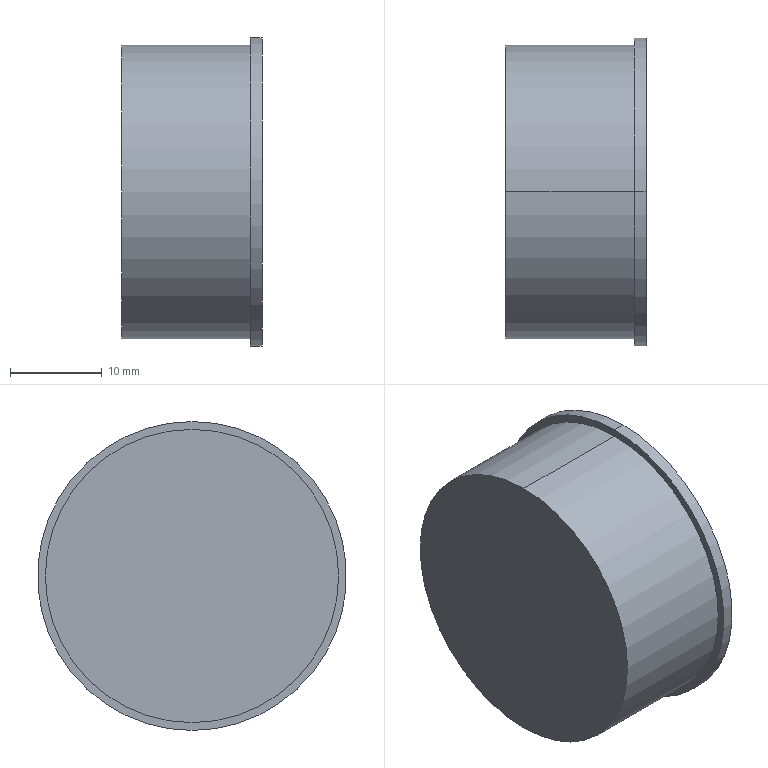Part | SolidWorks | features BaseBody 1 | 1 solid | 13 faces | box 15.3 x 33.7 x 33.7 mm | volume 12319 mm3 | cylinder 6 | cone 4 | plane 3 | commonest cylinder face diameters 4.5 x2 32 x2 33.7 x2
STEP:
#1=CARTESIAN_POINT('',(-209.5,-84.,82.771));
#2=VERTEX_POINT('',#1);
#3=CARTESIAN_POINT('',(-209.5,-84.,116.471));
#4=VERTEX_POINT('',#3);
#5=CARTESIAN_POINT('',(-209.5,-84.,99.621));
#6=DIRECTION('',(1.,0.,0.));
#7=DIRECTION('',(0.,0.,-1.));
#8=AXIS2_PLACEMENT_3D('',#5,#6,#7);
#9=CIRCLE('',#8,16.85);
#10=EDGE_CURVE('',#2,#4,#9,.T.);
#11=ORIENTED_EDGE('',*,*,#10,.T.);
#12=CARTESIAN_POINT('',(-208.2,-84.,116.471));
#13=VERTEX_POINT('',#12);
#14=CARTESIAN_POINT('',(-209.5,-84.,116.471));
#15=DIRECTION('',(1.,0.,0.));
#16=VECTOR('',#15,1000.);
#17=LINE('',#14,#16);
#18=EDGE_CURVE('',#4,#13,#17,.T.);
#19=ORIENTED_EDGE('',*,*,#18,.T.);
#20=CARTESIAN_POINT('',(-208.2,-84.,82.771));
#21=VERTEX_POINT('',#20);
#22=CARTESIAN_POINT('',(-208.2,-84.,99.621));
#23=DIRECTION('',(-1.,0.,0.));
#24=DIRECTION('',(0.,0.,-1.));
#25=AXIS2_PLACEMENT_3D('',#22,#23,#24);
#26=CIRCLE('',#25,16.85);
#27=EDGE_CURVE('',#13,#21,#26,.T.);
#28=ORIENTED_EDGE('',*,*,#27,.T.);
#29=CARTESIAN_POINT('',(-209.5,-84.,82.771));
#30=DIRECTION('',(1.,0.,0.));
#31=VECTOR('',#30,1000.);
#32=LINE('',#29,#31);
#33=EDGE_CURVE('',#2,#21,#32,.T.);
#34=ORIENTED_EDGE('',*,*,#33,.F.);
#35=EDGE_LOOP('',(#11,#19,#28,#34));
#36=FACE_OUTER_BOUND('',#35,.T.);
#37=CARTESIAN_POINT('',(-209.5,-84.,99.621));
#38=DIRECTION('',(1.,0.,0.));
#39=DIRECTION('',(0.,0.,-1.));
#40=AXIS2_PLACEMENT_3D('',#37,#38,#39);
#41=CYLINDRICAL_SURFACE('',#40,16.85);
#42=ADVANCED_FACE('',(#36),#41,.T.);
#43=CARTESIAN_POINT('',(-209.914,-86.25,99.621));
#44=VERTEX_POINT('',#43);
#45=CARTESIAN_POINT('',(-209.914,-84.,97.371));
#46=VERTEX_POINT('',#45);
#47=CARTESIAN_POINT('',(-209.914,-84.,99.621));
#48=DIRECTION('',(1.,0.,0.));
#49=DIRECTION('',(0.,0.3818,-0.9242));
#50=AXIS2_PLACEMENT_3D('',#47,#48,#49);
#51=CIRCLE('',#50,2.25);
#52=EDGE_CURVE('',#44,#46,#51,.T.);
#53=ORIENTED_EDGE('',*,*,#52,.F.);
#54=CARTESIAN_POINT('',(-208.2,-87.964,99.621));
#55=VERTEX_POINT('',#54);
#56=CARTESIAN_POINT('',(-208.2,-87.964,99.621));
#57=DIRECTION('',(0.7071,-0.7071,0.));
#58=VECTOR('',#57,1000.);
#59=LINE('',#56,#58);
#60=EDGE_CURVE('',#44,#55,#59,.T.);
#61=ORIENTED_EDGE('',*,*,#60,.T.);
#62=CARTESIAN_POINT('',(-208.2,-80.036,99.621));
#63=VERTEX_POINT('',#62);
#64=CARTESIAN_POINT('',(-208.2,-84.,99.621));
#65=DIRECTION('',(1.,0.,0.));
#66=DIRECTION('',(0.,1.,0.));
#67=AXIS2_PLACEMENT_3D('',#64,#65,#66);
#68=CIRCLE('',#67,3.964);
#69=EDGE_CURVE('',#55,#63,#68,.T.);
#70=ORIENTED_EDGE('',*,*,#69,.T.);
#71=CARTESIAN_POINT('',(-209.914,-81.75,99.621));
#72=VERTEX_POINT('',#71);
#73=CARTESIAN_POINT('',(-208.2,-80.036,99.621));
#74=DIRECTION('',(0.7071,0.7071,0.));
#75=VECTOR('',#74,1000.);
#76=LINE('',#73,#75);
#77=EDGE_CURVE('',#72,#63,#76,.T.);
#78=ORIENTED_EDGE('',*,*,#77,.F.);
#79=CARTESIAN_POINT('',(-209.914,-84.,99.621));
#80=DIRECTION('',(1.,0.,0.));
#81=DIRECTION('',(0.,0.3818,-0.9242));
#82=AXIS2_PLACEMENT_3D('',#79,#80,#81);
#83=CIRCLE('',#82,2.25);
#84=EDGE_CURVE('',#46,#72,#83,.T.);
#85=ORIENTED_EDGE('',*,*,#84,.F.);
#86=EDGE_LOOP('',(#53,#61,#70,#78,#85));
#87=FACE_OUTER_BOUND('',#86,.T.);
#88=CARTESIAN_POINT('',(-208.2,-84.,99.621));
#89=DIRECTION('',(1.,0.,0.));
#90=DIRECTION('',(0.,1.,0.));
#91=AXIS2_PLACEMENT_3D('',#88,#89,#90);
#92=CONICAL_SURFACE('',#91,3.964,0.7854);
#93=ADVANCED_FACE('',(#87),#92,.F.);
#94=CARTESIAN_POINT('',(-212.43,-84.,101.871));
#95=VERTEX_POINT('',#94);
#96=CARTESIAN_POINT('',(-212.43,-84.,97.371));
#97=VERTEX_POINT('',#96);
#98=CARTESIAN_POINT('',(-212.43,-84.,99.621));
#99=DIRECTION('',(1.,0.,0.));
#100=DIRECTION('',(0.,0.,-1.));
#101=AXIS2_PLACEMENT_3D('',#98,#99,#100);
#102=CIRCLE('',#101,2.25);
#103=EDGE_CURVE('',#95,#97,#102,.T.);
#104=ORIENTED_EDGE('',*,*,#103,.F.);
#105=CARTESIAN_POINT('',(-209.914,-84.,101.871));
#106=VERTEX_POINT('',#105);
#107=CARTESIAN_POINT('',(-208.2,-84.,101.871));
#108=DIRECTION('',(1.,0.,0.));
#109=VECTOR('',#108,1000.);
#110=LINE('',#107,#109);
#111=EDGE_CURVE('',#95,#106,#110,.T.);
#112=ORIENTED_EDGE('',*,*,#111,.T.);
#113=CARTESIAN_POINT('',(-209.914,-84.,99.621));
#114=DIRECTION('',(1.,0.,0.));
#115=DIRECTION('',(0.,0.3818,-0.9242));
#116=AXIS2_PLACEMENT_3D('',#113,#114,#115);
#117=CIRCLE('',#116,2.25);
#118=EDGE_CURVE('',#106,#44,#117,.T.);
#119=ORIENTED_EDGE('',*,*,#118,.T.);
#120=ORIENTED_EDGE('',*,*,#52,.T.);
#121=CARTESIAN_POINT('',(-208.2,-84.,97.371));
#122=DIRECTION('',(1.,0.,0.));
#123=VECTOR('',#122,1000.);
#124=LINE('',#121,#123);
#125=EDGE_CURVE('',#97,#46,#124,.T.);
#126=ORIENTED_EDGE('',*,*,#125,.F.);
#127=EDGE_LOOP('',(#104,#112,#119,#120,#126));
#128=FACE_OUTER_BOUND('',#127,.T.);
#129=CARTESIAN_POINT('',(-208.2,-84.,99.621));
#130=DIRECTION('',(1.,0.,0.));
#131=DIRECTION('',(0.,0.,-1.));
#132=AXIS2_PLACEMENT_3D('',#129,#130,#131);
#133=CYLINDRICAL_SURFACE('',#132,2.25);
#134=ADVANCED_FACE('',(#128),#133,.F.);
#135=CARTESIAN_POINT('',(-223.5,-84.,83.621));
#136=VERTEX_POINT('',#135);
#137=CARTESIAN_POINT('',(-223.5,-84.,115.621));
#138=VERTEX_POINT('',#137);
#139=CARTESIAN_POINT('',(-223.5,-84.,99.621));
#140=DIRECTION('',(1.,0.,0.));
#141=DIRECTION('',(0.,0.,-1.));
#142=AXIS2_PLACEMENT_3D('',#139,#140,#141);
#143=CIRCLE('',#142,16.);
#144=EDGE_CURVE('',#136,#138,#143,.T.);
#145=ORIENTED_EDGE('',*,*,#144,.T.);
#146=CARTESIAN_POINT('',(-209.5,-84.,115.621));
#147=VERTEX_POINT('',#146);
#148=CARTESIAN_POINT('',(-223.5,-84.,115.621));
#149=DIRECTION('',(1.,0.,0.));
#150=VECTOR('',#149,1000.);
#151=LINE('',#148,#150);
#152=EDGE_CURVE('',#138,#147,#151,.T.);
#153=ORIENTED_EDGE('',*,*,#152,.T.);
#154=CARTESIAN_POINT('',(-209.5,-84.,83.621));
#155=VERTEX_POINT('',#154);
#156=CARTESIAN_POINT('',(-209.5,-84.,99.621));
#157=DIRECTION('',(1.,0.,0.));
#158=DIRECTION('',(0.,0.,-1.));
#159=AXIS2_PLACEMENT_3D('',#156,#157,#158);
#160=CIRCLE('',#159,16.);
#161=EDGE_CURVE('',#155,#147,#160,.T.);
#162=ORIENTED_EDGE('',*,*,#161,.F.);
#163=CARTESIAN_POINT('',(-223.5,-84.,83.621));
#164=DIRECTION('',(1.,0.,0.));
#165=VECTOR('',#164,1000.);
#166=LINE('',#163,#165);
#167=EDGE_CURVE('',#136,#155,#166,.T.);
#168=ORIENTED_EDGE('',*,*,#167,.F.);
#169=EDGE_LOOP('',(#145,#153,#162,#168));
#170=FACE_OUTER_BOUND('',#169,.T.);
#171=CARTESIAN_POINT('',(-223.5,-84.,99.621));
#172=DIRECTION('',(1.,0.,0.));
#173=DIRECTION('',(0.,0.,-1.));
#174=AXIS2_PLACEMENT_3D('',#171,#172,#173);
#175=CYLINDRICAL_SURFACE('',#174,16.);
#176=ADVANCED_FACE('',(#170),#175,.T.);
#177=CARTESIAN_POINT('',(-213.782,-84.,99.621));
#178=VERTEX_POINT('',#177);
#179=CARTESIAN_POINT('',(-212.43,-84.,97.371));
#180=DIRECTION('',(0.515,0.,-0.8572));
#181=VECTOR('',#180,1000.);
#182=LINE('',#179,#181);
#183=EDGE_CURVE('',#178,#97,#182,.T.);
#184=ORIENTED_EDGE('',*,*,#183,.F.);
#185=CARTESIAN_POINT('',(-212.43,-84.,101.871));
#186=DIRECTION('',(0.515,0.,0.8572));
#187=VECTOR('',#186,1000.);
#188=LINE('',#185,#187);
#189=EDGE_CURVE('',#178,#95,#188,.T.);
#190=ORIENTED_EDGE('',*,*,#189,.T.);
#191=ORIENTED_EDGE('',*,*,#103,.T.);
#192=EDGE_LOOP('',(#184,#190,#191));
#193=FACE_OUTER_BOUND('',#192,.T.);
#194=CARTESIAN_POINT('',(-212.43,-84.,99.621));
#195=DIRECTION('',(1.,0.,0.));
#196=DIRECTION('',(0.,0.,-1.));
#197=AXIS2_PLACEMENT_3D('',#194,#195,#196);
#198=CONICAL_SURFACE('',#197,2.25,1.03);
#199=ADVANCED_FACE('',(#193),#198,.F.);
#200=CARTESIAN_POINT('',(-208.2,-84.,99.621));
#201=DIRECTION('',(-1.,0.,0.));
#202=DIRECTION('',(0.,0.,-1.));
#203=AXIS2_PLACEMENT_3D('',#200,#201,#202);
#204=CIRCLE('',#203,16.85);
#205=EDGE_CURVE('',#21,#13,#204,.T.);
#206=ORIENTED_EDGE('',*,*,#205,.F.);
#207=ORIENTED_EDGE('',*,*,#27,.F.);
#208=EDGE_LOOP('',(#206,#207));
#209=FACE_OUTER_BOUND('',#208,.T.);
#210=CARTESIAN_POINT('',(-208.2,-84.,99.621));
#211=DIRECTION('',(1.,0.,0.));
#212=DIRECTION('',(0.,1.,0.));
#213=AXIS2_PLACEMENT_3D('',#210,#211,#212);
#214=CIRCLE('',#213,3.964);
#215=EDGE_CURVE('',#63,#55,#214,.T.);
#216=ORIENTED_EDGE('',*,*,#215,.F.);
#217=ORIENTED_EDGE('',*,*,#69,.F.);
#218=EDGE_LOOP('',(#216,#217));
#219=FACE_BOUND('',#218,.T.);
#220=CARTESIAN_POINT('',(-208.2,-84.,99.621));
#221=DIRECTION('',(-1.,0.,0.));
#222=DIRECTION('',(0.,0.,1.));
#223=AXIS2_PLACEMENT_3D('',#220,#221,#222);
#224=PLANE('',#223);
#225=ADVANCED_FACE('',(#209,#219),#224,.F.);
#226=ORIENTED_EDGE('',*,*,#18,.F.);
#227=CARTESIAN_POINT('',(-209.5,-84.,99.621));
#228=DIRECTION('',(1.,0.,0.));
#229=DIRECTION('',(0.,0.,-1.));
#230=AXIS2_PLACEMENT_3D('',#227,#228,#229);
#231=CIRCLE('',#230,16.85);
#232=EDGE_CURVE('',#4,#2,#231,.T.);
#233=ORIENTED_EDGE('',*,*,#232,.T.);
#234=ORIENTED_EDGE('',*,*,#33,.T.);
#235=ORIENTED_EDGE('',*,*,#205,.T.);
#236=EDGE_LOOP('',(#226,#233,#234,#235));
#237=FACE_OUTER_BOUND('',#236,.T.);
#238=CARTESIAN_POINT('',(-209.5,-84.,99.621));
#239=DIRECTION('',(1.,0.,0.));
#240=DIRECTION('',(0.,0.,-1.));
#241=AXIS2_PLACEMENT_3D('',#238,#239,#240);
#242=CYLINDRICAL_SURFACE('',#241,16.85);
#243=ADVANCED_FACE('',(#237),#242,.T.);
#244=ORIENTED_EDGE('',*,*,#60,.F.);
#245=ORIENTED_EDGE('',*,*,#118,.F.);
#246=CARTESIAN_POINT('',(-209.914,-84.,99.621));
#247=DIRECTION('',(1.,0.,0.));
#248=DIRECTION('',(0.,0.3818,-0.9242));
#249=AXIS2_PLACEMENT_3D('',#246,#247,#248);
#250=CIRCLE('',#249,2.25);
#251=EDGE_CURVE('',#72,#106,#250,.T.);
#252=ORIENTED_EDGE('',*,*,#251,.F.);
#253=ORIENTED_EDGE('',*,*,#77,.T.);
#254=ORIENTED_EDGE('',*,*,#215,.T.);
#255=EDGE_LOOP('',(#244,#245,#252,#253,#254));
#256=FACE_OUTER_BOUND('',#255,.T.);
#257=CARTESIAN_POINT('',(-208.2,-84.,99.621));
#258=DIRECTION('',(1.,0.,0.));
#259=DIRECTION('',(0.,1.,0.));
#260=AXIS2_PLACEMENT_3D('',#257,#258,#259);
#261=CONICAL_SURFACE('',#260,3.964,0.7854);
#262=ADVANCED_FACE('',(#256),#261,.F.);
#263=ORIENTED_EDGE('',*,*,#161,.T.);
#264=CARTESIAN_POINT('',(-209.5,-84.,99.621));
#265=DIRECTION('',(1.,0.,0.));
#266=DIRECTION('',(0.,0.,-1.));
#267=AXIS2_PLACEMENT_3D('',#264,#265,#266);
#268=CIRCLE('',#267,16.);
#269=EDGE_CURVE('',#147,#155,#268,.T.);
#270=ORIENTED_EDGE('',*,*,#269,.T.);
#271=EDGE_LOOP('',(#263,#270));
#272=FACE_BOUND('',#271,.T.);
#273=ORIENTED_EDGE('',*,*,#10,.F.);
#274=ORIENTED_EDGE('',*,*,#232,.F.);
#275=EDGE_LOOP('',(#273,#274));
#276=FACE_OUTER_BOUND('',#275,.T.);
#277=CARTESIAN_POINT('',(-209.5,-84.,99.621));
#278=DIRECTION('',(-1.,0.,0.));
#279=DIRECTION('',(0.,0.,1.));
#280=AXIS2_PLACEMENT_3D('',#277,#278,#279);
#281=PLANE('',#280);
#282=ADVANCED_FACE('',(#272,#276),#281,.T.);
#283=ORIENTED_EDGE('',*,*,#111,.F.);
#284=CARTESIAN_POINT('',(-212.43,-84.,99.621));
#285=DIRECTION('',(1.,0.,0.));
#286=DIRECTION('',(0.,0.,-1.));
#287=AXIS2_PLACEMENT_3D('',#284,#285,#286);
#288=CIRCLE('',#287,2.25);
#289=EDGE_CURVE('',#97,#95,#288,.T.);
#290=ORIENTED_EDGE('',*,*,#289,.F.);
#291=ORIENTED_EDGE('',*,*,#125,.T.);
#292=ORIENTED_EDGE('',*,*,#84,.T.);
#293=ORIENTED_EDGE('',*,*,#251,.T.);
#294=EDGE_LOOP('',(#283,#290,#291,#292,#293));
#295=FACE_OUTER_BOUND('',#294,.T.);
#296=CARTESIAN_POINT('',(-208.2,-84.,99.621));
#297=DIRECTION('',(1.,0.,0.));
#298=DIRECTION('',(0.,0.,-1.));
#299=AXIS2_PLACEMENT_3D('',#296,#297,#298);
#300=CYLINDRICAL_SURFACE('',#299,2.25);
#301=ADVANCED_FACE('',(#295),#300,.F.);
#302=ORIENTED_EDGE('',*,*,#152,.F.);
#303=CARTESIAN_POINT('',(-223.5,-84.,99.621));
#304=DIRECTION('',(1.,0.,0.));
#305=DIRECTION('',(0.,0.,-1.));
#306=AXIS2_PLACEMENT_3D('',#303,#304,#305);
#307=CIRCLE('',#306,16.);
#308=EDGE_CURVE('',#138,#136,#307,.T.);
#309=ORIENTED_EDGE('',*,*,#308,.T.);
#310=ORIENTED_EDGE('',*,*,#167,.T.);
#311=ORIENTED_EDGE('',*,*,#269,.F.);
#312=EDGE_LOOP('',(#302,#309,#310,#311));
#313=FACE_OUTER_BOUND('',#312,.T.);
#314=CARTESIAN_POINT('',(-223.5,-84.,99.621));
#315=DIRECTION('',(1.,0.,0.));
#316=DIRECTION('',(0.,0.,-1.));
#317=AXIS2_PLACEMENT_3D('',#314,#315,#316);
#318=CYLINDRICAL_SURFACE('',#317,16.);
#319=ADVANCED_FACE('',(#313),#318,.T.);
#320=ORIENTED_EDGE('',*,*,#189,.F.);
#321=ORIENTED_EDGE('',*,*,#183,.T.);
#322=ORIENTED_EDGE('',*,*,#289,.T.);
#323=EDGE_LOOP('',(#320,#321,#322));
#324=FACE_OUTER_BOUND('',#323,.T.);
#325=CARTESIAN_POINT('',(-212.43,-84.,99.621));
#326=DIRECTION('',(1.,0.,0.));
#327=DIRECTION('',(0.,0.,-1.));
#328=AXIS2_PLACEMENT_3D('',#325,#326,#327);
#329=CONICAL_SURFACE('',#328,2.25,1.03);
#330=ADVANCED_FACE('',(#324),#329,.F.);
#331=ORIENTED_EDGE('',*,*,#144,.F.);
#332=ORIENTED_EDGE('',*,*,#308,.F.);
#333=EDGE_LOOP('',(#331,#332));
#334=FACE_OUTER_BOUND('',#333,.T.);
#335=CARTESIAN_POINT('',(-223.5,-84.,99.621));
#336=DIRECTION('',(-1.,0.,0.));
#337=DIRECTION('',(0.,0.,1.));
#338=AXIS2_PLACEMENT_3D('',#335,#336,#337);
#339=PLANE('',#338);
#340=ADVANCED_FACE('',(#334),#339,.T.);
#341=CLOSED_SHELL('',(#42,#93,#134,#176,#199,#225,#243,#262,#282,#301,#319,#330,#340));
#342=MANIFOLD_SOLID_BREP('',#341);
#343=CARTESIAN_POINT('',(0.,0.,0.));
#344=DIRECTION('',(0.,0.,1.));
#345=DIRECTION('',(1.,0.,0.));
#346=AXIS2_PLACEMENT_3D('',#343,#344,#345);
#347=(LENGTH_UNIT()NAMED_UNIT(*)SI_UNIT(.MILLI.,.METRE.));
#348=UNCERTAINTY_MEASURE_WITH_UNIT(LENGTH_MEASURE(0.00001),#347,'','');
#349=(NAMED_UNIT(*)PLANE_ANGLE_UNIT()SI_UNIT($,.RADIAN.));
#350=(NAMED_UNIT(*)SI_UNIT($,.STERADIAN.)SOLID_ANGLE_UNIT());
#351=(GEOMETRIC_REPRESENTATION_CONTEXT(3)GLOBAL_UNCERTAINTY_ASSIGNED_CONTEXT((#348))GLOBAL_UNIT_ASSIGNED_CONTEXT((#347,#349,#350))REPRESENTATION_CONTEXT('',''));
#352=ADVANCED_BREP_SHAPE_REPRESENTATION('',(#342,#346),#351);